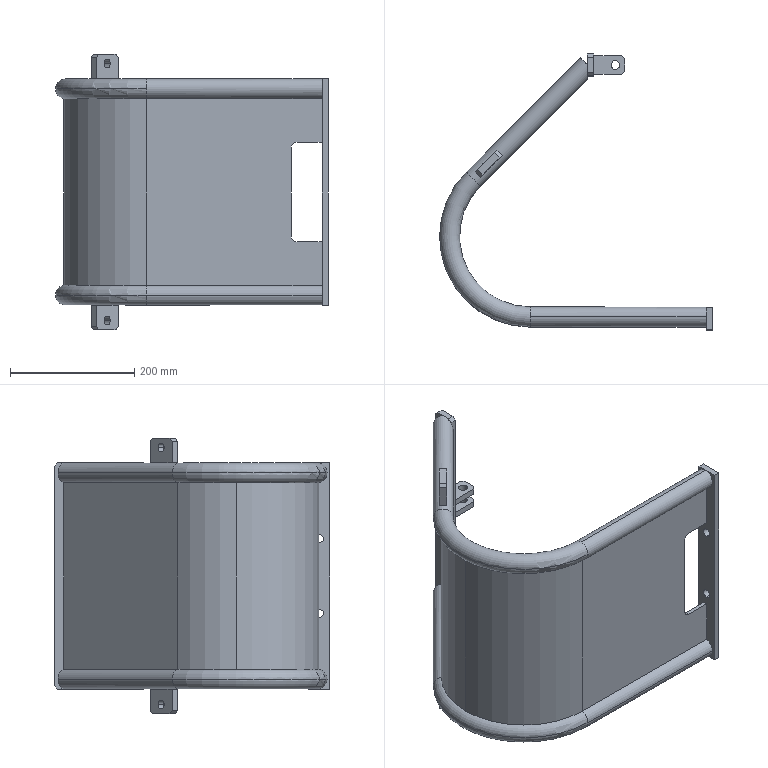Part | SolidWorks | features ICE 9, Chamfer 5, Sweep 2, BossThin 1 | 9 solids | 109 faces | box 439 x 443.772 x 444 mm | volume 2517725 mm3 | plane 67 | cylinder 34 | torus 8 | commonest cylinder face diameters 14 x12 22 x8 32 x8 20 x2 254 x2 266 x2